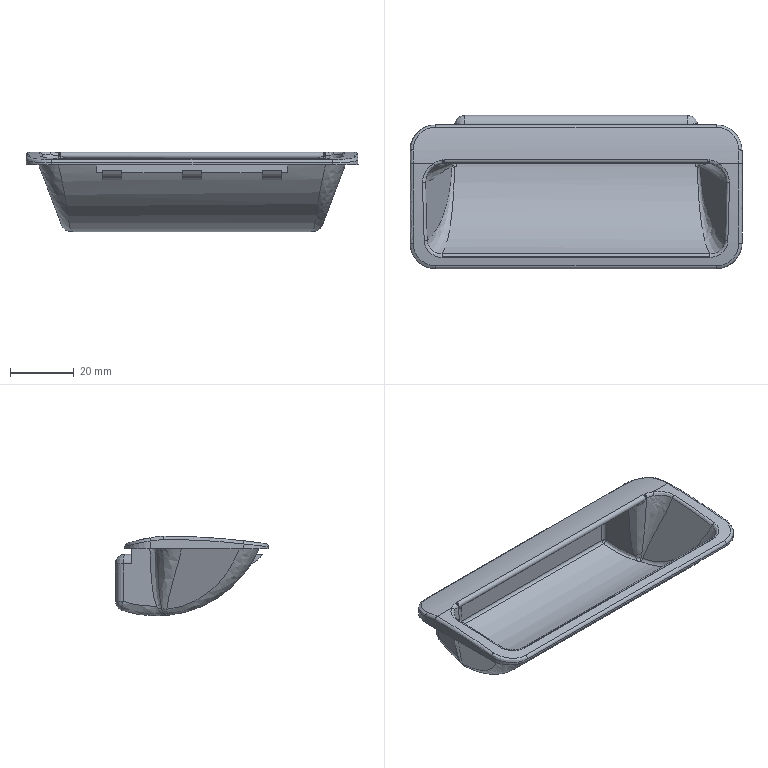Part | SolidWorks | features BaseBody 1 | 1 solid | 133 faces | box 104 x 48 x 25 mm | volume 19338 mm3 | spline 72 | cylinder 31 | plane 30 | commonest cylinder face diameters 2 x11 6 x6 16 x4 12 x3 4 x1 8 x1